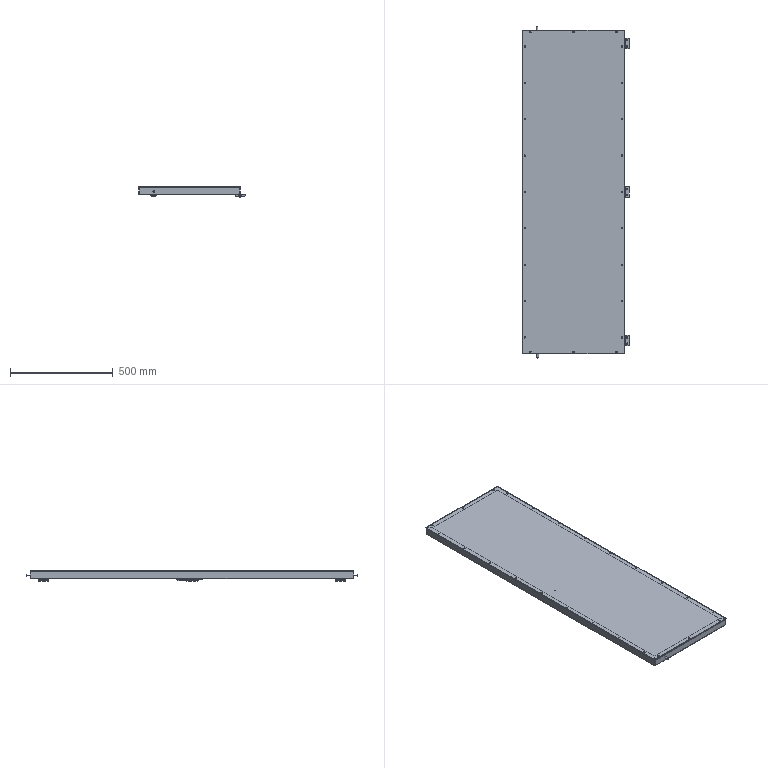Part | SolidWorks | 13 solids | 1434 faces | box 519.5 x 1618 x 50.5 mm | volume 4251711 mm3 | cylinder 623 | plane 564 | spline 194 | cone 53 | commonest cylinder face diameters 1 x144 5 x66 0.8 x52 6.5 x48 6.1 x46 6 x32